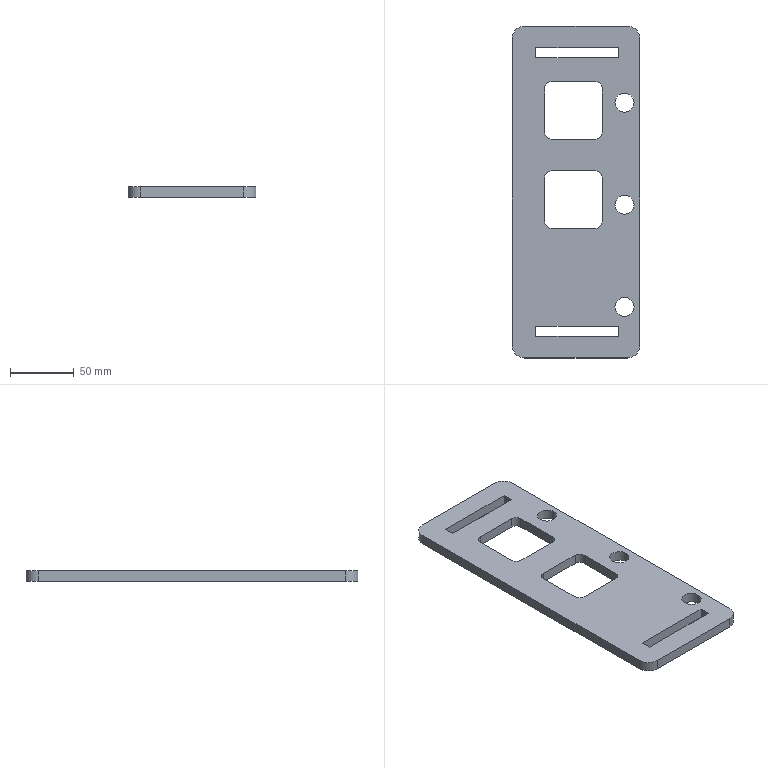Part | SolidWorks | features FlatPattern 1, SMBaseFlange 1, SheetMetal 1 | 1 solid | 40 faces | box 100 x 260 x 8 mm | volume 162695 mm3 | plane 22 | cylinder 18 | commonest cylinder face diameters 10 x8 15 x6 20 x4
STEP:
#1=CARTESIAN_POINT('',(-132.99,-115.,8.));
#2=VERTEX_POINT('',#1);
#3=CARTESIAN_POINT('',(-117.99,-115.,8.));
#4=VERTEX_POINT('',#3);
#5=CARTESIAN_POINT('',(-125.49,-115.,8.));
#6=DIRECTION('',(0.,0.,1.));
#7=DIRECTION('',(1.,0.,0.));
#8=AXIS2_PLACEMENT_3D('',#5,#6,#7);
#9=CIRCLE('',#8,7.5);
#10=EDGE_CURVE('',#2,#4,#9,.T.);
#11=ORIENTED_EDGE('',*,*,#10,.T.);
#12=CARTESIAN_POINT('',(-117.99,-115.,0.));
#13=VERTEX_POINT('',#12);
#14=CARTESIAN_POINT('',(-117.99,-115.,8.));
#15=DIRECTION('',(0.,0.,-1.));
#16=VECTOR('',#15,1000.);
#17=LINE('',#14,#16);
#18=EDGE_CURVE('',#4,#13,#17,.T.);
#19=ORIENTED_EDGE('',*,*,#18,.T.);
#20=CARTESIAN_POINT('',(-132.99,-115.,0.));
#21=VERTEX_POINT('',#20);
#22=CARTESIAN_POINT('',(-125.49,-115.,0.));
#23=DIRECTION('',(0.,0.,1.));
#24=DIRECTION('',(1.,0.,0.));
#25=AXIS2_PLACEMENT_3D('',#22,#23,#24);
#26=CIRCLE('',#25,7.5);
#27=EDGE_CURVE('',#21,#13,#26,.T.);
#28=ORIENTED_EDGE('',*,*,#27,.F.);
#29=CARTESIAN_POINT('',(-132.99,-115.,8.));
#30=DIRECTION('',(0.,0.,-1.));
#31=VECTOR('',#30,1000.);
#32=LINE('',#29,#31);
#33=EDGE_CURVE('',#2,#21,#32,.T.);
#34=ORIENTED_EDGE('',*,*,#33,.F.);
#35=EDGE_LOOP('',(#11,#19,#28,#34));
#36=FACE_OUTER_BOUND('',#35,.T.);
#37=CARTESIAN_POINT('',(-125.49,-115.,8.));
#38=DIRECTION('',(0.,0.,-1.));
#39=DIRECTION('',(-1.,0.,0.));
#40=AXIS2_PLACEMENT_3D('',#37,#38,#39);
#41=CYLINDRICAL_SURFACE('',#40,7.5);
#42=ADVANCED_FACE('',(#36),#41,.F.);
#43=CARTESIAN_POINT('',(-132.99,-195.,8.));
#44=VERTEX_POINT('',#43);
#45=CARTESIAN_POINT('',(-117.99,-195.,8.));
#46=VERTEX_POINT('',#45);
#47=CARTESIAN_POINT('',(-125.49,-195.,8.));
#48=DIRECTION('',(0.,0.,1.));
#49=DIRECTION('',(1.,0.,0.));
#50=AXIS2_PLACEMENT_3D('',#47,#48,#49);
#51=CIRCLE('',#50,7.5);
#52=EDGE_CURVE('',#44,#46,#51,.T.);
#53=ORIENTED_EDGE('',*,*,#52,.T.);
#54=CARTESIAN_POINT('',(-117.99,-195.,0.));
#55=VERTEX_POINT('',#54);
#56=CARTESIAN_POINT('',(-117.99,-195.,8.));
#57=DIRECTION('',(0.,0.,-1.));
#58=VECTOR('',#57,1000.);
#59=LINE('',#56,#58);
#60=EDGE_CURVE('',#46,#55,#59,.T.);
#61=ORIENTED_EDGE('',*,*,#60,.T.);
#62=CARTESIAN_POINT('',(-132.99,-195.,0.));
#63=VERTEX_POINT('',#62);
#64=CARTESIAN_POINT('',(-125.49,-195.,0.));
#65=DIRECTION('',(0.,0.,1.));
#66=DIRECTION('',(1.,0.,0.));
#67=AXIS2_PLACEMENT_3D('',#64,#65,#66);
#68=CIRCLE('',#67,7.5);
#69=EDGE_CURVE('',#63,#55,#68,.T.);
#70=ORIENTED_EDGE('',*,*,#69,.F.);
#71=CARTESIAN_POINT('',(-132.99,-195.,8.));
#72=DIRECTION('',(0.,0.,-1.));
#73=VECTOR('',#72,1000.);
#74=LINE('',#71,#73);
#75=EDGE_CURVE('',#44,#63,#74,.T.);
#76=ORIENTED_EDGE('',*,*,#75,.F.);
#77=EDGE_LOOP('',(#53,#61,#70,#76));
#78=FACE_OUTER_BOUND('',#77,.T.);
#79=CARTESIAN_POINT('',(-125.49,-195.,8.));
#80=DIRECTION('',(0.,0.,-1.));
#81=DIRECTION('',(-1.,0.,0.));
#82=AXIS2_PLACEMENT_3D('',#79,#80,#81);
#83=CYLINDRICAL_SURFACE('',#82,7.5);
#84=ADVANCED_FACE('',(#78),#83,.F.);
#85=CARTESIAN_POINT('',(-132.99,-275.,8.));
#86=VERTEX_POINT('',#85);
#87=CARTESIAN_POINT('',(-117.99,-275.,8.));
#88=VERTEX_POINT('',#87);
#89=CARTESIAN_POINT('',(-125.49,-275.,8.));
#90=DIRECTION('',(0.,0.,1.));
#91=DIRECTION('',(1.,0.,0.));
#92=AXIS2_PLACEMENT_3D('',#89,#90,#91);
#93=CIRCLE('',#92,7.5);
#94=EDGE_CURVE('',#86,#88,#93,.T.);
#95=ORIENTED_EDGE('',*,*,#94,.T.);
#96=CARTESIAN_POINT('',(-117.99,-275.,0.));
#97=VERTEX_POINT('',#96);
#98=CARTESIAN_POINT('',(-117.99,-275.,8.));
#99=DIRECTION('',(0.,0.,-1.));
#100=VECTOR('',#99,1000.);
#101=LINE('',#98,#100);
#102=EDGE_CURVE('',#88,#97,#101,.T.);
#103=ORIENTED_EDGE('',*,*,#102,.T.);
#104=CARTESIAN_POINT('',(-132.99,-275.,0.));
#105=VERTEX_POINT('',#104);
#106=CARTESIAN_POINT('',(-125.49,-275.,0.));
#107=DIRECTION('',(0.,0.,1.));
#108=DIRECTION('',(1.,0.,0.));
#109=AXIS2_PLACEMENT_3D('',#106,#107,#108);
#110=CIRCLE('',#109,7.5);
#111=EDGE_CURVE('',#105,#97,#110,.T.);
#112=ORIENTED_EDGE('',*,*,#111,.F.);
#113=CARTESIAN_POINT('',(-132.99,-275.,8.));
#114=DIRECTION('',(0.,0.,-1.));
#115=VECTOR('',#114,1000.);
#116=LINE('',#113,#115);
#117=EDGE_CURVE('',#86,#105,#116,.T.);
#118=ORIENTED_EDGE('',*,*,#117,.F.);
#119=EDGE_LOOP('',(#95,#103,#112,#118));
#120=FACE_OUTER_BOUND('',#119,.T.);
#121=CARTESIAN_POINT('',(-125.49,-275.,8.));
#122=DIRECTION('',(0.,0.,-1.));
#123=DIRECTION('',(-1.,0.,0.));
#124=AXIS2_PLACEMENT_3D('',#121,#122,#123);
#125=CYLINDRICAL_SURFACE('',#124,7.5);
#126=ADVANCED_FACE('',(#120),#125,.F.);
#127=ORIENTED_EDGE('',*,*,#52,.F.);
#128=CARTESIAN_POINT('',(-125.49,-195.,8.));
#129=DIRECTION('',(0.,0.,1.));
#130=DIRECTION('',(1.,0.,0.));
#131=AXIS2_PLACEMENT_3D('',#128,#129,#130);
#132=CIRCLE('',#131,7.5);
#133=EDGE_CURVE('',#46,#44,#132,.T.);
#134=ORIENTED_EDGE('',*,*,#133,.F.);
#135=EDGE_LOOP('',(#127,#134));
#136=FACE_BOUND('',#135,.T.);
#137=CARTESIAN_POINT('',(-213.472,-305.,8.));
#138=VERTEX_POINT('',#137);
#139=CARTESIAN_POINT('',(-203.472,-315.,8.));
#140=VERTEX_POINT('',#139);
#141=CARTESIAN_POINT('',(-203.472,-305.,8.));
#142=DIRECTION('',(0.,0.,1.));
#143=DIRECTION('',(1.,0.,0.));
#144=AXIS2_PLACEMENT_3D('',#141,#142,#143);
#145=CIRCLE('',#144,10.);
#146=EDGE_CURVE('',#138,#140,#145,.T.);
#147=ORIENTED_EDGE('',*,*,#146,.T.);
#148=CARTESIAN_POINT('',(-123.472,-315.,8.));
#149=VERTEX_POINT('',#148);
#150=CARTESIAN_POINT('',(-203.472,-315.,8.));
#151=DIRECTION('',(1.,0.,0.));
#152=VECTOR('',#151,1000.);
#153=LINE('',#150,#152);
#154=EDGE_CURVE('',#140,#149,#153,.T.);
#155=ORIENTED_EDGE('',*,*,#154,.T.);
#156=CARTESIAN_POINT('',(-113.472,-305.,8.));
#157=VERTEX_POINT('',#156);
#158=CARTESIAN_POINT('',(-123.472,-305.,8.));
#159=DIRECTION('',(0.,0.,1.));
#160=DIRECTION('',(1.,0.,0.));
#161=AXIS2_PLACEMENT_3D('',#158,#159,#160);
#162=CIRCLE('',#161,10.);
#163=EDGE_CURVE('',#149,#157,#162,.T.);
#164=ORIENTED_EDGE('',*,*,#163,.T.);
#165=CARTESIAN_POINT('',(-113.472,-65.,8.));
#166=VERTEX_POINT('',#165);
#167=CARTESIAN_POINT('',(-113.472,-65.,8.));
#168=DIRECTION('',(0.,1.,0.));
#169=VECTOR('',#168,1000.);
#170=LINE('',#167,#169);
#171=EDGE_CURVE('',#157,#166,#170,.T.);
#172=ORIENTED_EDGE('',*,*,#171,.T.);
#173=CARTESIAN_POINT('',(-123.472,-55.,8.));
#174=VERTEX_POINT('',#173);
#175=CARTESIAN_POINT('',(-123.472,-65.,8.));
#176=DIRECTION('',(0.,0.,1.));
#177=DIRECTION('',(-1.,0.,0.));
#178=AXIS2_PLACEMENT_3D('',#175,#176,#177);
#179=CIRCLE('',#178,10.);
#180=EDGE_CURVE('',#166,#174,#179,.T.);
#181=ORIENTED_EDGE('',*,*,#180,.T.);
#182=CARTESIAN_POINT('',(-203.472,-55.,8.));
#183=VERTEX_POINT('',#182);
#184=CARTESIAN_POINT('',(-203.472,-55.,8.));
#185=DIRECTION('',(-1.,0.,0.));
#186=VECTOR('',#185,1000.);
#187=LINE('',#184,#186);
#188=EDGE_CURVE('',#174,#183,#187,.T.);
#189=ORIENTED_EDGE('',*,*,#188,.T.);
#190=CARTESIAN_POINT('',(-213.472,-65.,8.));
#191=VERTEX_POINT('',#190);
#192=CARTESIAN_POINT('',(-203.472,-65.,8.));
#193=DIRECTION('',(0.,0.,1.));
#194=DIRECTION('',(1.,0.,0.));
#195=AXIS2_PLACEMENT_3D('',#192,#193,#194);
#196=CIRCLE('',#195,10.);
#197=EDGE_CURVE('',#183,#191,#196,.T.);
#198=ORIENTED_EDGE('',*,*,#197,.T.);
#199=CARTESIAN_POINT('',(-213.472,-65.,8.));
#200=DIRECTION('',(0.,-1.,0.));
#201=VECTOR('',#200,1000.);
#202=LINE('',#199,#201);
#203=EDGE_CURVE('',#191,#138,#202,.T.);
#204=ORIENTED_EDGE('',*,*,#203,.T.);
#205=EDGE_LOOP('',(#147,#155,#164,#172,#181,#189,#198,#204));
#206=FACE_OUTER_BOUND('',#205,.T.);
#207=ORIENTED_EDGE('',*,*,#94,.F.);
#208=CARTESIAN_POINT('',(-125.49,-275.,8.));
#209=DIRECTION('',(0.,0.,1.));
#210=DIRECTION('',(1.,0.,0.));
#211=AXIS2_PLACEMENT_3D('',#208,#209,#210);
#212=CIRCLE('',#211,7.5);
#213=EDGE_CURVE('',#88,#86,#212,.T.);
#214=ORIENTED_EDGE('',*,*,#213,.F.);
#215=EDGE_LOOP('',(#207,#214));
#216=FACE_BOUND('',#215,.T.);
#217=ORIENTED_EDGE('',*,*,#10,.F.);
#218=CARTESIAN_POINT('',(-125.49,-115.,8.));
#219=DIRECTION('',(0.,0.,1.));
#220=DIRECTION('',(1.,0.,0.));
#221=AXIS2_PLACEMENT_3D('',#218,#219,#220);
#222=CIRCLE('',#221,7.5);
#223=EDGE_CURVE('',#4,#2,#222,.T.);
#224=ORIENTED_EDGE('',*,*,#223,.F.);
#225=EDGE_LOOP('',(#217,#224));
#226=FACE_BOUND('',#225,.T.);
#227=CARTESIAN_POINT('',(-182.99,-143.5,8.));
#228=VERTEX_POINT('',#227);
#229=CARTESIAN_POINT('',(-147.99,-143.5,8.));
#230=VERTEX_POINT('',#229);
#231=CARTESIAN_POINT('',(-182.99,-143.5,8.));
#232=DIRECTION('',(1.,0.,0.));
#233=VECTOR('',#232,1000.);
#234=LINE('',#231,#233);
#235=EDGE_CURVE('',#228,#230,#234,.T.);
#236=ORIENTED_EDGE('',*,*,#235,.F.);
#237=CARTESIAN_POINT('',(-187.99,-138.5,8.));
#238=VERTEX_POINT('',#237);
#239=CARTESIAN_POINT('',(-182.99,-138.5,8.));
#240=DIRECTION('',(0.,0.,1.));
#241=DIRECTION('',(1.,0.,0.));
#242=AXIS2_PLACEMENT_3D('',#239,#240,#241);
#243=CIRCLE('',#242,5.);
#244=EDGE_CURVE('',#238,#228,#243,.T.);
#245=ORIENTED_EDGE('',*,*,#244,.F.);
#246=CARTESIAN_POINT('',(-187.99,-103.5,8.));
#247=VERTEX_POINT('',#246);
#248=CARTESIAN_POINT('',(-187.99,-103.5,8.));
#249=DIRECTION('',(0.,-1.,0.));
#250=VECTOR('',#249,1000.);
#251=LINE('',#248,#250);
#252=EDGE_CURVE('',#247,#238,#251,.T.);
#253=ORIENTED_EDGE('',*,*,#252,.F.);
#254=CARTESIAN_POINT('',(-182.99,-98.5,8.));
#255=VERTEX_POINT('',#254);
#256=CARTESIAN_POINT('',(-182.99,-103.5,8.));
#257=DIRECTION('',(0.,0.,1.));
#258=DIRECTION('',(1.,0.,0.));
#259=AXIS2_PLACEMENT_3D('',#256,#257,#258);
#260=CIRCLE('',#259,5.);
#261=EDGE_CURVE('',#255,#247,#260,.T.);
#262=ORIENTED_EDGE('',*,*,#261,.F.);
#263=CARTESIAN_POINT('',(-147.99,-98.5,8.));
#264=VERTEX_POINT('',#263);
#265=CARTESIAN_POINT('',(-182.99,-98.5,8.));
#266=DIRECTION('',(-1.,0.,0.));
#267=VECTOR('',#266,1000.);
#268=LINE('',#265,#267);
#269=EDGE_CURVE('',#264,#255,#268,.T.);
#270=ORIENTED_EDGE('',*,*,#269,.F.);
#271=CARTESIAN_POINT('',(-142.99,-103.5,8.));
#272=VERTEX_POINT('',#271);
#273=CARTESIAN_POINT('',(-147.99,-103.5,8.));
#274=DIRECTION('',(0.,0.,1.));
#275=DIRECTION('',(-1.,0.,0.));
#276=AXIS2_PLACEMENT_3D('',#273,#274,#275);
#277=CIRCLE('',#276,5.);
#278=EDGE_CURVE('',#272,#264,#277,.T.);
#279=ORIENTED_EDGE('',*,*,#278,.F.);
#280=CARTESIAN_POINT('',(-142.99,-138.5,8.));
#281=VERTEX_POINT('',#280);
#282=CARTESIAN_POINT('',(-142.99,-103.5,8.));
#283=DIRECTION('',(0.,1.,0.));
#284=VECTOR('',#283,1000.);
#285=LINE('',#282,#284);
#286=EDGE_CURVE('',#281,#272,#285,.T.);
#287=ORIENTED_EDGE('',*,*,#286,.F.);
#288=CARTESIAN_POINT('',(-147.99,-138.5,8.));
#289=DIRECTION('',(0.,0.,1.));
#290=DIRECTION('',(1.,0.,0.));
#291=AXIS2_PLACEMENT_3D('',#288,#289,#290);
#292=CIRCLE('',#291,5.);
#293=EDGE_CURVE('',#230,#281,#292,.T.);
#294=ORIENTED_EDGE('',*,*,#293,.F.);
#295=EDGE_LOOP('',(#236,#245,#253,#262,#270,#279,#287,#294));
#296=FACE_BOUND('',#295,.T.);
#297=CARTESIAN_POINT('',(-182.99,-213.5,8.));
#298=VERTEX_POINT('',#297);
#299=CARTESIAN_POINT('',(-147.99,-213.5,8.));
#300=VERTEX_POINT('',#299);
#301=CARTESIAN_POINT('',(-182.99,-213.5,8.));
#302=DIRECTION('',(1.,0.,0.));
#303=VECTOR('',#302,1000.);
#304=LINE('',#301,#303);
#305=EDGE_CURVE('',#298,#300,#304,.T.);
#306=ORIENTED_EDGE('',*,*,#305,.F.);
#307=CARTESIAN_POINT('',(-187.99,-208.5,8.));
#308=VERTEX_POINT('',#307);
#309=CARTESIAN_POINT('',(-182.99,-208.5,8.));
#310=DIRECTION('',(0.,0.,1.));
#311=DIRECTION('',(1.,0.,0.));
#312=AXIS2_PLACEMENT_3D('',#309,#310,#311);
#313=CIRCLE('',#312,5.);
#314=EDGE_CURVE('',#308,#298,#313,.T.);
#315=ORIENTED_EDGE('',*,*,#314,.F.);
#316=CARTESIAN_POINT('',(-187.99,-173.5,8.));
#317=VERTEX_POINT('',#316);
#318=CARTESIAN_POINT('',(-187.99,-173.5,8.));
#319=DIRECTION('',(0.,-1.,0.));
#320=VECTOR('',#319,1000.);
#321=LINE('',#318,#320);
#322=EDGE_CURVE('',#317,#308,#321,.T.);
#323=ORIENTED_EDGE('',*,*,#322,.F.);
#324=CARTESIAN_POINT('',(-182.99,-168.5,8.));
#325=VERTEX_POINT('',#324);
#326=CARTESIAN_POINT('',(-182.99,-173.5,8.));
#327=DIRECTION('',(0.,0.,1.));
#328=DIRECTION('',(1.,0.,0.));
#329=AXIS2_PLACEMENT_3D('',#326,#327,#328);
#330=CIRCLE('',#329,5.);
#331=EDGE_CURVE('',#325,#317,#330,.T.);
#332=ORIENTED_EDGE('',*,*,#331,.F.);
#333=CARTESIAN_POINT('',(-147.99,-168.5,8.));
#334=VERTEX_POINT('',#333);
#335=CARTESIAN_POINT('',(-182.99,-168.5,8.));
#336=DIRECTION('',(-1.,0.,0.));
#337=VECTOR('',#336,1000.);
#338=LINE('',#335,#337);
#339=EDGE_CURVE('',#334,#325,#338,.T.);
#340=ORIENTED_EDGE('',*,*,#339,.F.);
#341=CARTESIAN_POINT('',(-142.99,-173.5,8.));
#342=VERTEX_POINT('',#341);
#343=CARTESIAN_POINT('',(-147.99,-173.5,8.));
#344=DIRECTION('',(0.,0.,1.));
#345=DIRECTION('',(-1.,0.,0.));
#346=AXIS2_PLACEMENT_3D('',#343,#344,#345);
#347=CIRCLE('',#346,5.);
#348=EDGE_CURVE('',#342,#334,#347,.T.);
#349=ORIENTED_EDGE('',*,*,#348,.F.);
#350=CARTESIAN_POINT('',(-142.99,-208.5,8.));
#351=VERTEX_POINT('',#350);
#352=CARTESIAN_POINT('',(-142.99,-173.5,8.));
#353=DIRECTION('',(0.,1.,0.));
#354=VECTOR('',#353,1000.);
#355=LINE('',#352,#354);
#356=EDGE_CURVE('',#351,#342,#355,.T.);
#357=ORIENTED_EDGE('',*,*,#356,.F.);
#358=CARTESIAN_POINT('',(-147.99,-208.5,8.));
#359=DIRECTION('',(0.,0.,1.));
#360=DIRECTION('',(1.,0.,0.));
#361=AXIS2_PLACEMENT_3D('',#358,#359,#360);
#362=CIRCLE('',#361,5.);
#363=EDGE_CURVE('',#300,#351,#362,.T.);
#364=ORIENTED_EDGE('',*,*,#363,.F.);
#365=EDGE_LOOP('',(#306,#315,#323,#332,#340,#349,#357,#364));
#366=FACE_BOUND('',#365,.T.);
#367=CARTESIAN_POINT('',(-130.006,-290.,8.));
#368=VERTEX_POINT('',#367);
#369=CARTESIAN_POINT('',(-195.006,-290.,8.));
#370=VERTEX_POINT('',#369);
#371=CARTESIAN_POINT('',(-130.006,-290.,8.));
#372=DIRECTION('',(-1.,0.,0.));
#373=VECTOR('',#372,1000.);
#374=LINE('',#371,#373);
#375=EDGE_CURVE('',#368,#370,#374,.T.);
#376=ORIENTED_EDGE('',*,*,#375,.F.);
#377=CARTESIAN_POINT('',(-130.006,-298.,8.));
#378=VERTEX_POINT('',#377);
#379=CARTESIAN_POINT('',(-130.006,-298.,8.));
#380=DIRECTION('',(0.,1.,0.));
#381=VECTOR('',#380,1000.);
#382=LINE('',#379,#381);
#383=EDGE_CURVE('',#378,#368,#382,.T.);
#384=ORIENTED_EDGE('',*,*,#383,.F.);
#385=CARTESIAN_POINT('',(-195.006,-298.,8.));
#386=VERTEX_POINT('',#385);
#387=CARTESIAN_POINT('',(-130.006,-298.,8.));
#388=DIRECTION('',(1.,0.,0.));
#389=VECTOR('',#388,1000.);
#390=LINE('',#387,#389);
#391=EDGE_CURVE('',#386,#378,#390,.T.);
#392=ORIENTED_EDGE('',*,*,#391,.F.);
#393=CARTESIAN_POINT('',(-195.006,-298.,8.));
#394=DIRECTION('',(0.,-1.,0.));
#395=VECTOR('',#394,1000.);
#396=LINE('',#393,#395);
#397=EDGE_CURVE('',#370,#386,#396,.T.);
#398=ORIENTED_EDGE('',*,*,#397,.F.);
#399=EDGE_LOOP('',(#376,#384,#392,#398));
#400=FACE_BOUND('',#399,.T.);
#401=CARTESIAN_POINT('',(-130.006,-72.,8.));
#402=VERTEX_POINT('',#401);
#403=CARTESIAN_POINT('',(-195.006,-72.,8.));
#404=VERTEX_POINT('',#403);
#405=CARTESIAN_POINT('',(-130.006,-72.,8.));
#406=DIRECTION('',(-1.,0.,0.));
#407=VECTOR('',#406,1000.);
#408=LINE('',#405,#407);
#409=EDGE_CURVE('',#402,#404,#408,.T.);
#410=ORIENTED_EDGE('',*,*,#409,.F.);
#411=CARTESIAN_POINT('',(-130.006,-80.,8.));
#412=VERTEX_POINT('',#411);
#413=CARTESIAN_POINT('',(-130.006,-72.,8.));
#414=DIRECTION('',(0.,1.,0.));
#415=VECTOR('',#414,1000.);
#416=LINE('',#413,#415);
#417=EDGE_CURVE('',#412,#402,#416,.T.);
#418=ORIENTED_EDGE('',*,*,#417,.F.);
#419=CARTESIAN_POINT('',(-195.006,-80.,8.));
#420=VERTEX_POINT('',#419);
#421=CARTESIAN_POINT('',(-130.006,-80.,8.));
#422=DIRECTION('',(1.,0.,0.));
#423=VECTOR('',#422,1000.);
#424=LINE('',#421,#423);
#425=EDGE_CURVE('',#420,#412,#424,.T.);
#426=ORIENTED_EDGE('',*,*,#425,.F.);
#427=CARTESIAN_POINT('',(-195.006,-72.,8.));
#428=DIRECTION('',(0.,-1.,0.));
#429=VECTOR('',#428,1000.);
#430=LINE('',#427,#429);
#431=EDGE_CURVE('',#404,#420,#430,.T.);
#432=ORIENTED_EDGE('',*,*,#431,.F.);
#433=EDGE_LOOP('',(#410,#418,#426,#432));
#434=FACE_BOUND('',#433,.T.);
#435=CARTESIAN_POINT('',(-203.472,-305.,8.));
#436=DIRECTION('',(0.,0.,1.));
#437=DIRECTION('',(1.,0.,0.));
#438=AXIS2_PLACEMENT_3D('',#435,#436,#437);
#439=PLANE('',#438);
#440=ADVANCED_FACE('',(#136,#206,#216,#226,#296,#366,#400,#434),#439,.T.);
#441=CARTESIAN_POINT('',(-130.006,-298.,0.));
#442=VERTEX_POINT('',#441);
#443=CARTESIAN_POINT('',(-130.006,-290.,0.));
#444=VERTEX_POINT('',#443);
#445=CARTESIAN_POINT('',(-130.006,-298.,0.));
#446=DIRECTION('',(0.,1.,0.));
#447=VECTOR('',#446,1000.);
#448=LINE('',#445,#447);
#449=EDGE_CURVE('',#442,#444,#448,.T.);
#450=ORIENTED_EDGE('',*,*,#449,.T.);
#451=CARTESIAN_POINT('',(-195.006,-290.,0.));
#452=VERTEX_POINT('',#451);
#453=CARTESIAN_POINT('',(-130.006,-290.,0.));
#454=DIRECTION('',(-1.,0.,0.));
#455=VECTOR('',#454,1000.);
#456=LINE('',#453,#455);
#457=EDGE_CURVE('',#444,#452,#456,.T.);
#458=ORIENTED_EDGE('',*,*,#457,.T.);
#459=CARTESIAN_POINT('',(-195.006,-298.,0.));
#460=VERTEX_POINT('',#459);
#461=CARTESIAN_POINT('',(-195.006,-298.,0.));
#462=DIRECTION('',(0.,-1.,0.));
#463=VECTOR('',#462,1000.);
#464=LINE('',#461,#463);
#465=EDGE_CURVE('',#452,#460,#464,.T.);
#466=ORIENTED_EDGE('',*,*,#465,.T.);
#467=CARTESIAN_POINT('',(-130.006,-298.,0.));
#468=DIRECTION('',(1.,0.,0.));
#469=VECTOR('',#468,1000.);
#470=LINE('',#467,#469);
#471=EDGE_CURVE('',#460,#442,#470,.T.);
#472=ORIENTED_EDGE('',*,*,#471,.T.);
#473=EDGE_LOOP('',(#450,#458,#466,#472));
#474=FACE_BOUND('',#473,.T.);
#475=CARTESIAN_POINT('',(-187.99,-138.5,0.));
#476=VERTEX_POINT('',#475);
#477=CARTESIAN_POINT('',(-182.99,-143.5,0.));
#478=VERTEX_POINT('',#477);
#479=CARTESIAN_POINT('',(-182.99,-138.5,0.));
#480=DIRECTION('',(0.,0.,1.));
#481=DIRECTION('',(1.,0.,0.));
#482=AXIS2_PLACEMENT_3D('',#479,#480,#481);
#483=CIRCLE('',#482,5.);
#484=EDGE_CURVE('',#476,#478,#483,.T.);
#485=ORIENTED_EDGE('',*,*,#484,.T.);
#486=CARTESIAN_POINT('',(-147.99,-143.5,0.));
#487=VERTEX_POINT('',#486);
#488=CARTESIAN_POINT('',(-182.99,-143.5,0.));
#489=DIRECTION('',(1.,0.,0.));
#490=VECTOR('',#489,1000.);
#491=LINE('',#488,#490);
#492=EDGE_CURVE('',#478,#487,#491,.T.);
#493=ORIENTED_EDGE('',*,*,#492,.T.);
#494=CARTESIAN_POINT('',(-142.99,-138.5,0.));
#495=VERTEX_POINT('',#494);
#496=CARTESIAN_POINT('',(-147.99,-138.5,0.));
#497=DIRECTION('',(0.,0.,1.));
#498=DIRECTION('',(1.,0.,0.));
#499=AXIS2_PLACEMENT_3D('',#496,#497,#498);
#500=CIRCLE('',#499,5.);
#501=EDGE_CURVE('',#487,#495,#500,.T.);
#502=ORIENTED_EDGE('',*,*,#501,.T.);
#503=CARTESIAN_POINT('',(-142.99,-103.5,0.));
#504=VERTEX_POINT('',#503);
#505=CARTESIAN_POINT('',(-142.99,-103.5,0.));
#506=DIRECTION('',(0.,1.,0.));
#507=VECTOR('',#506,1000.);
#508=LINE('',#505,#507);
#509=EDGE_CURVE('',#495,#504,#508,.T.);
#510=ORIENTED_EDGE('',*,*,#509,.T.);
#511=CARTESIAN_POINT('',(-147.99,-98.5,0.));
#512=VERTEX_POINT('',#511);
#513=CARTESIAN_POINT('',(-147.99,-103.5,0.));
#514=DIRECTION('',(0.,0.,1.));
#515=DIRECTION('',(-1.,0.,0.));
#516=AXIS2_PLACEMENT_3D('',#513,#514,#515);
#517=CIRCLE('',#516,5.);
#518=EDGE_CURVE('',#504,#512,#517,.T.);
#519=ORIENTED_EDGE('',*,*,#518,.T.);
#520=CARTESIAN_POINT('',(-182.99,-98.5,0.));
#521=VERTEX_POINT('',#520);
#522=CARTESIAN_POINT('',(-182.99,-98.5,0.));
#523=DIRECTION('',(-1.,0.,0.));
#524=VECTOR('',#523,1000.);
#525=LINE('',#522,#524);
#526=EDGE_CURVE('',#512,#521,#525,.T.);
#527=ORIENTED_EDGE('',*,*,#526,.T.);
#528=CARTESIAN_POINT('',(-187.99,-103.5,0.));
#529=VERTEX_POINT('',#528);
#530=CARTESIAN_POINT('',(-182.99,-103.5,0.));
#531=DIRECTION('',(0.,0.,1.));
#532=DIRECTION('',(1.,0.,0.));
#533=AXIS2_PLACEMENT_3D('',#530,#531,#532);
#534=CIRCLE('',#533,5.);
#535=EDGE_CURVE('',#521,#529,#534,.T.);
#536=ORIENTED_EDGE('',*,*,#535,.T.);
#537=CARTESIAN_POINT('',(-187.99,-103.5,0.));
#538=DIRECTION('',(0.,-1.,0.));
#539=VECTOR('',#538,1000.);
#540=LINE('',#537,#539);
#541=EDGE_CURVE('',#529,#476,#540,.T.);
#542=ORIENTED_EDGE('',*,*,#541,.T.);
#543=EDGE_LOOP('',(#485,#493,#502,#510,#519,#527,#536,#542));
#544=FACE_BOUND('',#543,.T.);
#545=CARTESIAN_POINT('',(-213.472,-305.,0.));
#546=VERTEX_POINT('',#545);
#547=CARTESIAN_POINT('',(-203.472,-315.,0.));
#548=VERTEX_POINT('',#547);
#549=CARTESIAN_POINT('',(-203.472,-305.,0.));
#550=DIRECTION('',(0.,0.,1.));
#551=DIRECTION('',(1.,0.,0.));
#552=AXIS2_PLACEMENT_3D('',#549,#550,#551);
#553=CIRCLE('',#552,10.);
#554=EDGE_CURVE('',#546,#548,#553,.T.);
#555=ORIENTED_EDGE('',*,*,#554,.F.);
#556=CARTESIAN_POINT('',(-213.472,-65.,0.));
#557=VERTEX_POINT('',#556);
#558=CARTESIAN_POINT('',(-213.472,-65.,0.));
#559=DIRECTION('',(0.,-1.,0.));
#560=VECTOR('',#559,1000.);
#561=LINE('',#558,#560);
#562=EDGE_CURVE('',#557,#546,#561,.T.);
#563=ORIENTED_EDGE('',*,*,#562,.F.);
#564=CARTESIAN_POINT('',(-203.472,-55.,0.));
#565=VERTEX_POINT('',#564);
#566=CARTESIAN_POINT('',(-203.472,-65.,0.));
#567=DIRECTION('',(0.,0.,1.));
#568=DIRECTION('',(1.,0.,0.));
#569=AXIS2_PLACEMENT_3D('',#566,#567,#568);
#570=CIRCLE('',#569,10.);
#571=EDGE_CURVE('',#565,#557,#570,.T.);
#572=ORIENTED_EDGE('',*,*,#571,.F.);
#573=CARTESIAN_POINT('',(-123.472,-55.,0.));
#574=VERTEX_POINT('',#573);
#575=CARTESIAN_POINT('',(-203.472,-55.,0.));
#576=DIRECTION('',(-1.,0.,0.));
#577=VECTOR('',#576,1000.);
#578=LINE('',#575,#577);
#579=EDGE_CURVE('',#574,#565,#578,.T.);
#580=ORIENTED_EDGE('',*,*,#579,.F.);
#581=CARTESIAN_POINT('',(-113.472,-65.,0.));
#582=VERTEX_POINT('',#581);
#583=CARTESIAN_POINT('',(-123.472,-65.,0.));
#584=DIRECTION('',(0.,0.,1.));
#585=DIRECTION('',(-1.,0.,0.));
#586=AXIS2_PLACEMENT_3D('',#583,#584,#585);
#587=CIRCLE('',#586,10.);
#588=EDGE_CURVE('',#582,#574,#587,.T.);
#589=ORIENTED_EDGE('',*,*,#588,.F.);
#590=CARTESIAN_POINT('',(-113.472,-305.,0.));
#591=VERTEX_POINT('',#590);
#592=CARTESIAN_POINT('',(-113.472,-65.,0.));
#593=DIRECTION('',(0.,1.,0.));
#594=VECTOR('',#593,1000.);
#595=LINE('',#592,#594);
#596=EDGE_CURVE('',#591,#582,#595,.T.);
#597=ORIENTED_EDGE('',*,*,#596,.F.);
#598=CARTESIAN_POINT('',(-123.472,-315.,0.));
#599=VERTEX_POINT('',#598);
#600=CARTESIAN_POINT('',(-123.472,-305.,0.));
#601=DIRECTION('',(0.,0.,1.));
#602=DIRECTION('',(1.,0.,0.));
#603=AXIS2_PLACEMENT_3D('',#600,#601,#602);
#604=CIRCLE('',#603,10.);
#605=EDGE_CURVE('',#599,#591,#604,.T.);
#606=ORIENTED_EDGE('',*,*,#605,.F.);
#607=CARTESIAN_POINT('',(-203.472,-315.,0.));
#608=DIRECTION('',(1.,0.,0.));
#609=VECTOR('',#608,1000.);
#610=LINE('',#607,#609);
#611=EDGE_CURVE('',#548,#599,#610,.T.);
#612=ORIENTED_EDGE('',*,*,#611,.F.);
#613=EDGE_LOOP('',(#555,#563,#572,#580,#589,#597,#606,#612));
#614=FACE_OUTER_BOUND('',#613,.T.);
#615=ORIENTED_EDGE('',*,*,#111,.T.);
#616=CARTESIAN_POINT('',(-125.49,-275.,0.));
#617=DIRECTION('',(0.,0.,1.));
#618=DIRECTION('',(1.,0.,0.));
#619=AXIS2_PLACEMENT_3D('',#616,#617,#618);
#620=CIRCLE('',#619,7.5);
#621=EDGE_CURVE('',#97,#105,#620,.T.);
#622=ORIENTED_EDGE('',*,*,#621,.T.);
#623=EDGE_LOOP('',(#615,#622));
#624=FACE_BOUND('',#623,.T.);
#625=ORIENTED_EDGE('',*,*,#69,.T.);
#626=CARTESIAN_POINT('',(-125.49,-195.,0.));
#627=DIRECTION('',(0.,0.,1.));
#628=DIRECTION('',(1.,0.,0.));
#629=AXIS2_PLACEMENT_3D('',#626,#627,#628);
#630=CIRCLE('',#629,7.5);
#631=EDGE_CURVE('',#55,#63,#630,.T.);
#632=ORIENTED_EDGE('',*,*,#631,.T.);
#633=EDGE_LOOP('',(#625,#632));
#634=FACE_BOUND('',#633,.T.);
#635=ORIENTED_EDGE('',*,*,#27,.T.);
#636=CARTESIAN_POINT('',(-125.49,-115.,0.));
#637=DIRECTION('',(0.,0.,1.));
#638=DIRECTION('',(1.,0.,0.));
#639=AXIS2_PLACEMENT_3D('',#636,#637,#638);
#640=CIRCLE('',#639,7.5);
#641=EDGE_CURVE('',#13,#21,#640,.T.);
#642=ORIENTED_EDGE('',*,*,#641,.T.);
#643=EDGE_LOOP('',(#635,#642));
#644=FACE_BOUND('',#643,.T.);
#645=CARTESIAN_POINT('',(-187.99,-208.5,0.));
#646=VERTEX_POINT('',#645);
#647=CARTESIAN_POINT('',(-182.99,-213.5,0.));
#648=VERTEX_POINT('',#647);
#649=CARTESIAN_POINT('',(-182.99,-208.5,0.));
#650=DIRECTION('',(0.,0.,1.));
#651=DIRECTION('',(1.,0.,0.));
#652=AXIS2_PLACEMENT_3D('',#649,#650,#651);
#653=CIRCLE('',#652,5.);
#654=EDGE_CURVE('',#646,#648,#653,.T.);
#655=ORIENTED_EDGE('',*,*,#654,.T.);
#656=CARTESIAN_POINT('',(-147.99,-213.5,0.));
#657=VERTEX_POINT('',#656);
#658=CARTESIAN_POINT('',(-182.99,-213.5,0.));
#659=DIRECTION('',(1.,0.,0.));
#660=VECTOR('',#659,1000.);
#661=LINE('',#658,#660);
#662=EDGE_CURVE('',#648,#657,#661,.T.);
#663=ORIENTED_EDGE('',*,*,#662,.T.);
#664=CARTESIAN_POINT('',(-142.99,-208.5,0.));
#665=VERTEX_POINT('',#664);
#666=CARTESIAN_POINT('',(-147.99,-208.5,0.));
#667=DIRECTION('',(0.,0.,1.));
#668=DIRECTION('',(1.,0.,0.));
#669=AXIS2_PLACEMENT_3D('',#666,#667,#668);
#670=CIRCLE('',#669,5.);
#671=EDGE_CURVE('',#657,#665,#670,.T.);
#672=ORIENTED_EDGE('',*,*,#671,.T.);
#673=CARTESIAN_POINT('',(-142.99,-173.5,0.));
#674=VERTEX_POINT('',#673);
#675=CARTESIAN_POINT('',(-142.99,-173.5,0.));
#676=DIRECTION('',(0.,1.,0.));
#677=VECTOR('',#676,1000.);
#678=LINE('',#675,#677);
#679=EDGE_CURVE('',#665,#674,#678,.T.);
#680=ORIENTED_EDGE('',*,*,#679,.T.);
#681=CARTESIAN_POINT('',(-147.99,-168.5,0.));
#682=VERTEX_POINT('',#681);
#683=CARTESIAN_POINT('',(-147.99,-173.5,0.));
#684=DIRECTION('',(0.,0.,1.));
#685=DIRECTION('',(-1.,0.,0.));
#686=AXIS2_PLACEMENT_3D('',#683,#684,#685);
#687=CIRCLE('',#686,5.);
#688=EDGE_CURVE('',#674,#682,#687,.T.);
#689=ORIENTED_EDGE('',*,*,#688,.T.);
#690=CARTESIAN_POINT('',(-182.99,-168.5,0.));
#691=VERTEX_POINT('',#690);
#692=CARTESIAN_POINT('',(-182.99,-168.5,0.));
#693=DIRECTION('',(-1.,0.,0.));
#694=VECTOR('',#693,1000.);
#695=LINE('',#692,#694);
#696=EDGE_CURVE('',#682,#691,#695,.T.);
#697=ORIENTED_EDGE('',*,*,#696,.T.);
#698=CARTESIAN_POINT('',(-187.99,-173.5,0.));
#699=VERTEX_POINT('',#698);
#700=CARTESIAN_POINT('',(-182.99,-173.5,0.));
#701=DIRECTION('',(0.,0.,1.));
#702=DIRECTION('',(1.,0.,0.));
#703=AXIS2_PLACEMENT_3D('',#700,#701,#702);
#704=CIRCLE('',#703,5.);
#705=EDGE_CURVE('',#691,#699,#704,.T.);
#706=ORIENTED_EDGE('',*,*,#705,.T.);
#707=CARTESIAN_POINT('',(-187.99,-173.5,0.));
#708=DIRECTION('',(0.,-1.,0.));
#709=VECTOR('',#708,1000.);
#710=LINE('',#707,#709);
#711=EDGE_CURVE('',#699,#646,#710,.T.);
#712=ORIENTED_EDGE('',*,*,#711,.T.);
#713=EDGE_LOOP('',(#655,#663,#672,#680,#689,#697,#706,#712));
#714=FACE_BOUND('',#713,.T.);
#715=CARTESIAN_POINT('',(-130.006,-80.,0.));
#716=VERTEX_POINT('',#715);
#717=CARTESIAN_POINT('',(-130.006,-72.,0.));
#718=VERTEX_POINT('',#717);
#719=CARTESIAN_POINT('',(-130.006,-72.,0.));
#720=DIRECTION('',(0.,1.,0.));
#721=VECTOR('',#720,1000.);
#722=LINE('',#719,#721);
#723=EDGE_CURVE('',#716,#718,#722,.T.);
#724=ORIENTED_EDGE('',*,*,#723,.T.);
#725=CARTESIAN_POINT('',(-195.006,-72.,0.));
#726=VERTEX_POINT('',#725);
#727=CARTESIAN_POINT('',(-130.006,-72.,0.));
#728=DIRECTION('',(-1.,0.,0.));
#729=VECTOR('',#728,1000.);
#730=LINE('',#727,#729);
#731=EDGE_CURVE('',#718,#726,#730,.T.);
#732=ORIENTED_EDGE('',*,*,#731,.T.);
#733=CARTESIAN_POINT('',(-195.006,-80.,0.));
#734=VERTEX_POINT('',#733);
#735=CARTESIAN_POINT('',(-195.006,-72.,0.));
#736=DIRECTION('',(0.,-1.,0.));
#737=VECTOR('',#736,1000.);
#738=LINE('',#735,#737);
#739=EDGE_CURVE('',#726,#734,#738,.T.);
#740=ORIENTED_EDGE('',*,*,#739,.T.);
#741=CARTESIAN_POINT('',(-130.006,-80.,0.));
#742=DIRECTION('',(1.,0.,0.));
#743=VECTOR('',#742,1000.);
#744=LINE('',#741,#743);
#745=EDGE_CURVE('',#734,#716,#744,.T.);
#746=ORIENTED_EDGE('',*,*,#745,.T.);
#747=EDGE_LOOP('',(#724,#732,#740,#746));
#748=FACE_BOUND('',#747,.T.);
#749=CARTESIAN_POINT('',(-203.472,-305.,0.));
#750=DIRECTION('',(0.,0.,1.));
#751=DIRECTION('',(1.,0.,0.));
#752=AXIS2_PLACEMENT_3D('',#749,#750,#751);
#753=PLANE('',#752);
#754=ADVANCED_FACE('',(#474,#544,#614,#624,#634,#644,#714,#748),#753,.F.);
#755=ORIENTED_EDGE('',*,*,#554,.T.);
#756=CARTESIAN_POINT('',(-203.472,-315.,8.));
#757=DIRECTION('',(0.,0.,-1.));
#758=VECTOR('',#757,1000.);
#759=LINE('',#756,#758);
#760=EDGE_CURVE('',#140,#548,#759,.T.);
#761=ORIENTED_EDGE('',*,*,#760,.F.);
#762=ORIENTED_EDGE('',*,*,#146,.F.);
#763=CARTESIAN_POINT('',(-213.472,-305.,8.));
#764=DIRECTION('',(0.,0.,-1.));
#765=VECTOR('',#764,1000.);
#766=LINE('',#763,#765);
#767=EDGE_CURVE('',#138,#546,#766,.T.);
#768=ORIENTED_EDGE('',*,*,#767,.T.);
#769=EDGE_LOOP('',(#755,#761,#762,#768));
#770=FACE_OUTER_BOUND('',#769,.T.);
#771=CARTESIAN_POINT('',(-203.472,-305.,8.));
#772=DIRECTION('',(0.,0.,-1.));
#773=DIRECTION('',(-1.,0.,0.));
#774=AXIS2_PLACEMENT_3D('',#771,#772,#773);
#775=CYLINDRICAL_SURFACE('',#774,10.);
#776=ADVANCED_FACE('',(#770),#775,.T.);
#777=ORIENTED_EDGE('',*,*,#611,.T.);
#778=CARTESIAN_POINT('',(-123.472,-315.,8.));
#779=DIRECTION('',(0.,0.,-1.));
#780=VECTOR('',#779,1000.);
#781=LINE('',#778,#780);
#782=EDGE_CURVE('',#149,#599,#781,.T.);
#783=ORIENTED_EDGE('',*,*,#782,.F.);
#784=ORIENTED_EDGE('',*,*,#154,.F.);
#785=ORIENTED_EDGE('',*,*,#760,.T.);
#786=EDGE_LOOP('',(#777,#783,#784,#785));
#787=FACE_OUTER_BOUND('',#786,.T.);
#788=CARTESIAN_POINT('',(-203.472,-315.,8.));
#789=DIRECTION('',(0.,1.,0.));
#790=DIRECTION('',(0.,0.,1.));
#791=AXIS2_PLACEMENT_3D('',#788,#789,#790);
#792=PLANE('',#791);
#793=ADVANCED_FACE('',(#787),#792,.F.);
#794=ORIENTED_EDGE('',*,*,#605,.T.);
#795=CARTESIAN_POINT('',(-113.472,-305.,8.));
#796=DIRECTION('',(0.,0.,-1.));
#797=VECTOR('',#796,1000.);
#798=LINE('',#795,#797);
#799=EDGE_CURVE('',#157,#591,#798,.T.);
#800=ORIENTED_EDGE('',*,*,#799,.F.);
#801=ORIENTED_EDGE('',*,*,#163,.F.);
#802=ORIENTED_EDGE('',*,*,#782,.T.);
#803=EDGE_LOOP('',(#794,#800,#801,#802));
#804=FACE_OUTER_BOUND('',#803,.T.);
#805=CARTESIAN_POINT('',(-123.472,-305.,8.));
#806=DIRECTION('',(0.,0.,-1.));
#807=DIRECTION('',(-1.,0.,0.));
#808=AXIS2_PLACEMENT_3D('',#805,#806,#807);
#809=CYLINDRICAL_SURFACE('',#808,10.);
#810=ADVANCED_FACE('',(#804),#809,.T.);
#811=ORIENTED_EDGE('',*,*,#596,.T.);
#812=CARTESIAN_POINT('',(-113.472,-65.,8.));
#813=DIRECTION('',(0.,0.,-1.));
#814=VECTOR('',#813,1000.);
#815=LINE('',#812,#814);
#816=EDGE_CURVE('',#166,#582,#815,.T.);
#817=ORIENTED_EDGE('',*,*,#816,.F.);
#818=ORIENTED_EDGE('',*,*,#171,.F.);
#819=ORIENTED_EDGE('',*,*,#799,.T.);
#820=EDGE_LOOP('',(#811,#817,#818,#819));
#821=FACE_OUTER_BOUND('',#820,.T.);
#822=CARTESIAN_POINT('',(-113.472,-65.,8.));
#823=DIRECTION('',(-1.,0.,0.));
#824=DIRECTION('',(0.,-1.,0.));
#825=AXIS2_PLACEMENT_3D('',#822,#823,#824);
#826=PLANE('',#825);
#827=ADVANCED_FACE('',(#821),#826,.F.);
#828=ORIENTED_EDGE('',*,*,#588,.T.);
#829=CARTESIAN_POINT('',(-123.472,-55.,8.));
#830=DIRECTION('',(0.,0.,-1.));
#831=VECTOR('',#830,1000.);
#832=LINE('',#829,#831);
#833=EDGE_CURVE('',#174,#574,#832,.T.);
#834=ORIENTED_EDGE('',*,*,#833,.F.);
#835=ORIENTED_EDGE('',*,*,#180,.F.);
#836=ORIENTED_EDGE('',*,*,#816,.T.);
#837=EDGE_LOOP('',(#828,#834,#835,#836));
#838=FACE_OUTER_BOUND('',#837,.T.);
#839=CARTESIAN_POINT('',(-123.472,-65.,8.));
#840=DIRECTION('',(0.,0.,-1.));
#841=DIRECTION('',(-1.,0.,0.));
#842=AXIS2_PLACEMENT_3D('',#839,#840,#841);
#843=CYLINDRICAL_SURFACE('',#842,10.);
#844=ADVANCED_FACE('',(#838),#843,.T.);
#845=ORIENTED_EDGE('',*,*,#579,.T.);
#846=CARTESIAN_POINT('',(-203.472,-55.,8.));
#847=DIRECTION('',(0.,0.,-1.));
#848=VECTOR('',#847,1000.);
#849=LINE('',#846,#848);
#850=EDGE_CURVE('',#183,#565,#849,.T.);
#851=ORIENTED_EDGE('',*,*,#850,.F.);
#852=ORIENTED_EDGE('',*,*,#188,.F.);
#853=ORIENTED_EDGE('',*,*,#833,.T.);
#854=EDGE_LOOP('',(#845,#851,#852,#853));
#855=FACE_OUTER_BOUND('',#854,.T.);
#856=CARTESIAN_POINT('',(-203.472,-55.,8.));
#857=DIRECTION('',(0.,-1.,0.));
#858=DIRECTION('',(1.,0.,0.));
#859=AXIS2_PLACEMENT_3D('',#856,#857,#858);
#860=PLANE('',#859);
#861=ADVANCED_FACE('',(#855),#860,.F.);
#862=ORIENTED_EDGE('',*,*,#571,.T.);
#863=CARTESIAN_POINT('',(-213.472,-65.,8.));
#864=DIRECTION('',(0.,0.,-1.));
#865=VECTOR('',#864,1000.);
#866=LINE('',#863,#865);
#867=EDGE_CURVE('',#191,#557,#866,.T.);
#868=ORIENTED_EDGE('',*,*,#867,.F.);
#869=ORIENTED_EDGE('',*,*,#197,.F.);
#870=ORIENTED_EDGE('',*,*,#850,.T.);
#871=EDGE_LOOP('',(#862,#868,#869,#870));
#872=FACE_OUTER_BOUND('',#871,.T.);
#873=CARTESIAN_POINT('',(-203.472,-65.,8.));
#874=DIRECTION('',(0.,0.,-1.));
#875=DIRECTION('',(-1.,0.,0.));
#876=AXIS2_PLACEMENT_3D('',#873,#874,#875);
#877=CYLINDRICAL_SURFACE('',#876,10.);
#878=ADVANCED_FACE('',(#872),#877,.T.);
#879=ORIENTED_EDGE('',*,*,#562,.T.);
#880=ORIENTED_EDGE('',*,*,#767,.F.);
#881=ORIENTED_EDGE('',*,*,#203,.F.);
#882=ORIENTED_EDGE('',*,*,#867,.T.);
#883=EDGE_LOOP('',(#879,#880,#881,#882));
#884=FACE_OUTER_BOUND('',#883,.T.);
#885=CARTESIAN_POINT('',(-213.472,-65.,8.));
#886=DIRECTION('',(1.,0.,0.));
#887=DIRECTION('',(0.,1.,0.));
#888=AXIS2_PLACEMENT_3D('',#885,#886,#887);
#889=PLANE('',#888);
#890=ADVANCED_FACE('',(#884),#889,.F.);
#891=ORIENTED_EDGE('',*,*,#102,.F.);
#892=ORIENTED_EDGE('',*,*,#213,.T.);
#893=ORIENTED_EDGE('',*,*,#117,.T.);
#894=ORIENTED_EDGE('',*,*,#621,.F.);
#895=EDGE_LOOP('',(#891,#892,#893,#894));
#896=FACE_OUTER_BOUND('',#895,.T.);
#897=CARTESIAN_POINT('',(-125.49,-275.,8.));
#898=DIRECTION('',(0.,0.,-1.));
#899=DIRECTION('',(-1.,0.,0.));
#900=AXIS2_PLACEMENT_3D('',#897,#898,#899);
#901=CYLINDRICAL_SURFACE('',#900,7.5);
#902=ADVANCED_FACE('',(#896),#901,.F.);
#903=ORIENTED_EDGE('',*,*,#60,.F.);
#904=ORIENTED_EDGE('',*,*,#133,.T.);
#905=ORIENTED_EDGE('',*,*,#75,.T.);
#906=ORIENTED_EDGE('',*,*,#631,.F.);
#907=EDGE_LOOP('',(#903,#904,#905,#906));
#908=FACE_OUTER_BOUND('',#907,.T.);
#909=CARTESIAN_POINT('',(-125.49,-195.,8.));
#910=DIRECTION('',(0.,0.,-1.));
#911=DIRECTION('',(-1.,0.,0.));
#912=AXIS2_PLACEMENT_3D('',#909,#910,#911);
#913=CYLINDRICAL_SURFACE('',#912,7.5);
#914=ADVANCED_FACE('',(#908),#913,.F.);
#915=ORIENTED_EDGE('',*,*,#18,.F.);
#916=ORIENTED_EDGE('',*,*,#223,.T.);
#917=ORIENTED_EDGE('',*,*,#33,.T.);
#918=ORIENTED_EDGE('',*,*,#641,.F.);
#919=EDGE_LOOP('',(#915,#916,#917,#918));
#920=FACE_OUTER_BOUND('',#919,.T.);
#921=CARTESIAN_POINT('',(-125.49,-115.,8.));
#922=DIRECTION('',(0.,0.,-1.));
#923=DIRECTION('',(-1.,0.,0.));
#924=AXIS2_PLACEMENT_3D('',#921,#922,#923);
#925=CYLINDRICAL_SURFACE('',#924,7.5);
#926=ADVANCED_FACE('',(#920),#925,.F.);
#927=ORIENTED_EDGE('',*,*,#484,.F.);
#928=CARTESIAN_POINT('',(-187.99,-138.5,8.));
#929=DIRECTION('',(0.,0.,-1.));
#930=VECTOR('',#929,1000.);
#931=LINE('',#928,#930);
#932=EDGE_CURVE('',#238,#476,#931,.T.);
#933=ORIENTED_EDGE('',*,*,#932,.F.);
#934=ORIENTED_EDGE('',*,*,#244,.T.);
#935=CARTESIAN_POINT('',(-182.99,-143.5,8.));
#936=DIRECTION('',(0.,0.,-1.));
#937=VECTOR('',#936,1000.);
#938=LINE('',#935,#937);
#939=EDGE_CURVE('',#228,#478,#938,.T.);
#940=ORIENTED_EDGE('',*,*,#939,.T.);
#941=EDGE_LOOP('',(#927,#933,#934,#940));
#942=FACE_OUTER_BOUND('',#941,.T.);
#943=CARTESIAN_POINT('',(-182.99,-138.5,8.));
#944=DIRECTION('',(0.,0.,-1.));
#945=DIRECTION('',(-1.,0.,0.));
#946=AXIS2_PLACEMENT_3D('',#943,#944,#945);
#947=CYLINDRICAL_SURFACE('',#946,5.);
#948=ADVANCED_FACE('',(#942),#947,.F.);
#949=ORIENTED_EDGE('',*,*,#492,.F.);
#950=ORIENTED_EDGE('',*,*,#939,.F.);
#951=ORIENTED_EDGE('',*,*,#235,.T.);
#952=CARTESIAN_POINT('',(-147.99,-143.5,8.));
#953=DIRECTION('',(0.,0.,-1.));
#954=VECTOR('',#953,1000.);
#955=LINE('',#952,#954);
#956=EDGE_CURVE('',#230,#487,#955,.T.);
#957=ORIENTED_EDGE('',*,*,#956,.T.);
#958=EDGE_LOOP('',(#949,#950,#951,#957));
#959=FACE_OUTER_BOUND('',#958,.T.);
#960=CARTESIAN_POINT('',(-182.99,-143.5,8.));
#961=DIRECTION('',(0.,1.,0.));
#962=DIRECTION('',(0.,0.,1.));
#963=AXIS2_PLACEMENT_3D('',#960,#961,#962);
#964=PLANE('',#963);
#965=ADVANCED_FACE('',(#959),#964,.T.);
#966=ORIENTED_EDGE('',*,*,#501,.F.);
#967=ORIENTED_EDGE('',*,*,#956,.F.);
#968=ORIENTED_EDGE('',*,*,#293,.T.);
#969=CARTESIAN_POINT('',(-142.99,-138.5,8.));
#970=DIRECTION('',(0.,0.,-1.));
#971=VECTOR('',#970,1000.);
#972=LINE('',#969,#971);
#973=EDGE_CURVE('',#281,#495,#972,.T.);
#974=ORIENTED_EDGE('',*,*,#973,.T.);
#975=EDGE_LOOP('',(#966,#967,#968,#974));
#976=FACE_OUTER_BOUND('',#975,.T.);
#977=CARTESIAN_POINT('',(-147.99,-138.5,8.));
#978=DIRECTION('',(0.,0.,-1.));
#979=DIRECTION('',(-1.,0.,0.));
#980=AXIS2_PLACEMENT_3D('',#977,#978,#979);
#981=CYLINDRICAL_SURFACE('',#980,5.);
#982=ADVANCED_FACE('',(#976),#981,.F.);
#983=ORIENTED_EDGE('',*,*,#509,.F.);
#984=ORIENTED_EDGE('',*,*,#973,.F.);
#985=ORIENTED_EDGE('',*,*,#286,.T.);
#986=CARTESIAN_POINT('',(-142.99,-103.5,8.));
#987=DIRECTION('',(0.,0.,-1.));
#988=VECTOR('',#987,1000.);
#989=LINE('',#986,#988);
#990=EDGE_CURVE('',#272,#504,#989,.T.);
#991=ORIENTED_EDGE('',*,*,#990,.T.);
#992=EDGE_LOOP('',(#983,#984,#985,#991));
#993=FACE_OUTER_BOUND('',#992,.T.);
#994=CARTESIAN_POINT('',(-142.99,-103.5,8.));
#995=DIRECTION('',(-1.,0.,0.));
#996=DIRECTION('',(0.,0.,1.));
#997=AXIS2_PLACEMENT_3D('',#994,#995,#996);
#998=PLANE('',#997);
#999=ADVANCED_FACE('',(#993),#998,.T.);
#1000=ORIENTED_EDGE('',*,*,#518,.F.);
#1001=ORIENTED_EDGE('',*,*,#990,.F.);
#1002=ORIENTED_EDGE('',*,*,#278,.T.);
#1003=CARTESIAN_POINT('',(-147.99,-98.5,8.));
#1004=DIRECTION('',(0.,0.,-1.));
#1005=VECTOR('',#1004,1000.);
#1006=LINE('',#1003,#1005);
#1007=EDGE_CURVE('',#264,#512,#1006,.T.);
#1008=ORIENTED_EDGE('',*,*,#1007,.T.);
#1009=EDGE_LOOP('',(#1000,#1001,#1002,#1008));
#1010=FACE_OUTER_BOUND('',#1009,.T.);
#1011=CARTESIAN_POINT('',(-147.99,-103.5,8.));
#1012=DIRECTION('',(0.,0.,-1.));
#1013=DIRECTION('',(-1.,0.,0.));
#1014=AXIS2_PLACEMENT_3D('',#1011,#1012,#1013);
#1015=CYLINDRICAL_SURFACE('',#1014,5.);
#1016=ADVANCED_FACE('',(#1010),#1015,.F.);
#1017=ORIENTED_EDGE('',*,*,#526,.F.);
#1018=ORIENTED_EDGE('',*,*,#1007,.F.);
#1019=ORIENTED_EDGE('',*,*,#269,.T.);
#1020=CARTESIAN_POINT('',(-182.99,-98.5,8.));
#1021=DIRECTION('',(0.,0.,-1.));
#1022=VECTOR('',#1021,1000.);
#1023=LINE('',#1020,#1022);
#1024=EDGE_CURVE('',#255,#521,#1023,.T.);
#1025=ORIENTED_EDGE('',*,*,#1024,.T.);
#1026=EDGE_LOOP('',(#1017,#1018,#1019,#1025));
#1027=FACE_OUTER_BOUND('',#1026,.T.);
#1028=CARTESIAN_POINT('',(-182.99,-98.5,8.));
#1029=DIRECTION('',(0.,-1.,0.));
#1030=DIRECTION('',(0.,0.,-1.));
#1031=AXIS2_PLACEMENT_3D('',#1028,#1029,#1030);
#1032=PLANE('',#1031);
#1033=ADVANCED_FACE('',(#1027),#1032,.T.);
#1034=ORIENTED_EDGE('',*,*,#535,.F.);
#1035=ORIENTED_EDGE('',*,*,#1024,.F.);
#1036=ORIENTED_EDGE('',*,*,#261,.T.);
#1037=CARTESIAN_POINT('',(-187.99,-103.5,8.));
#1038=DIRECTION('',(0.,0.,-1.));
#1039=VECTOR('',#1038,1000.);
#1040=LINE('',#1037,#1039);
#1041=EDGE_CURVE('',#247,#529,#1040,.T.);
#1042=ORIENTED_EDGE('',*,*,#1041,.T.);
#1043=EDGE_LOOP('',(#1034,#1035,#1036,#1042));
#1044=FACE_OUTER_BOUND('',#1043,.T.);
#1045=CARTESIAN_POINT('',(-182.99,-103.5,8.));
#1046=DIRECTION('',(0.,0.,-1.));
#1047=DIRECTION('',(-1.,0.,0.));
#1048=AXIS2_PLACEMENT_3D('',#1045,#1046,#1047);
#1049=CYLINDRICAL_SURFACE('',#1048,5.);
#1050=ADVANCED_FACE('',(#1044),#1049,.F.);
#1051=ORIENTED_EDGE('',*,*,#541,.F.);
#1052=ORIENTED_EDGE('',*,*,#1041,.F.);
#1053=ORIENTED_EDGE('',*,*,#252,.T.);
#1054=ORIENTED_EDGE('',*,*,#932,.T.);
#1055=EDGE_LOOP('',(#1051,#1052,#1053,#1054));
#1056=FACE_OUTER_BOUND('',#1055,.T.);
#1057=CARTESIAN_POINT('',(-187.99,-103.5,8.));
#1058=DIRECTION('',(1.,0.,0.));
#1059=DIRECTION('',(0.,0.,-1.));
#1060=AXIS2_PLACEMENT_3D('',#1057,#1058,#1059);
#1061=PLANE('',#1060);
#1062=ADVANCED_FACE('',(#1056),#1061,.T.);
#1063=ORIENTED_EDGE('',*,*,#654,.F.);
#1064=CARTESIAN_POINT('',(-187.99,-208.5,8.));
#1065=DIRECTION('',(0.,0.,-1.));
#1066=VECTOR('',#1065,1000.);
#1067=LINE('',#1064,#1066);
#1068=EDGE_CURVE('',#308,#646,#1067,.T.);
#1069=ORIENTED_EDGE('',*,*,#1068,.F.);
#1070=ORIENTED_EDGE('',*,*,#314,.T.);
#1071=CARTESIAN_POINT('',(-182.99,-213.5,8.));
#1072=DIRECTION('',(0.,0.,-1.));
#1073=VECTOR('',#1072,1000.);
#1074=LINE('',#1071,#1073);
#1075=EDGE_CURVE('',#298,#648,#1074,.T.);
#1076=ORIENTED_EDGE('',*,*,#1075,.T.);
#1077=EDGE_LOOP('',(#1063,#1069,#1070,#1076));
#1078=FACE_OUTER_BOUND('',#1077,.T.);
#1079=CARTESIAN_POINT('',(-182.99,-208.5,8.));
#1080=DIRECTION('',(0.,0.,-1.));
#1081=DIRECTION('',(-1.,0.,0.));
#1082=AXIS2_PLACEMENT_3D('',#1079,#1080,#1081);
#1083=CYLINDRICAL_SURFACE('',#1082,5.);
#1084=ADVANCED_FACE('',(#1078),#1083,.F.);
#1085=ORIENTED_EDGE('',*,*,#662,.F.);
#1086=ORIENTED_EDGE('',*,*,#1075,.F.);
#1087=ORIENTED_EDGE('',*,*,#305,.T.);
#1088=CARTESIAN_POINT('',(-147.99,-213.5,8.));
#1089=DIRECTION('',(0.,0.,-1.));
#1090=VECTOR('',#1089,1000.);
#1091=LINE('',#1088,#1090);
#1092=EDGE_CURVE('',#300,#657,#1091,.T.);
#1093=ORIENTED_EDGE('',*,*,#1092,.T.);
#1094=EDGE_LOOP('',(#1085,#1086,#1087,#1093));
#1095=FACE_OUTER_BOUND('',#1094,.T.);
#1096=CARTESIAN_POINT('',(-182.99,-213.5,8.));
#1097=DIRECTION('',(0.,1.,0.));
#1098=DIRECTION('',(0.,0.,1.));
#1099=AXIS2_PLACEMENT_3D('',#1096,#1097,#1098);
#1100=PLANE('',#1099);
#1101=ADVANCED_FACE('',(#1095),#1100,.T.);
#1102=ORIENTED_EDGE('',*,*,#671,.F.);
#1103=ORIENTED_EDGE('',*,*,#1092,.F.);
#1104=ORIENTED_EDGE('',*,*,#363,.T.);
#1105=CARTESIAN_POINT('',(-142.99,-208.5,8.));
#1106=DIRECTION('',(0.,0.,-1.));
#1107=VECTOR('',#1106,1000.);
#1108=LINE('',#1105,#1107);
#1109=EDGE_CURVE('',#351,#665,#1108,.T.);
#1110=ORIENTED_EDGE('',*,*,#1109,.T.);
#1111=EDGE_LOOP('',(#1102,#1103,#1104,#1110));
#1112=FACE_OUTER_BOUND('',#1111,.T.);
#1113=CARTESIAN_POINT('',(-147.99,-208.5,8.));
#1114=DIRECTION('',(0.,0.,-1.));
#1115=DIRECTION('',(-1.,0.,0.));
#1116=AXIS2_PLACEMENT_3D('',#1113,#1114,#1115);
#1117=CYLINDRICAL_SURFACE('',#1116,5.);
#1118=ADVANCED_FACE('',(#1112),#1117,.F.);
#1119=ORIENTED_EDGE('',*,*,#679,.F.);
#1120=ORIENTED_EDGE('',*,*,#1109,.F.);
#1121=ORIENTED_EDGE('',*,*,#356,.T.);
#1122=CARTESIAN_POINT('',(-142.99,-173.5,8.));
#1123=DIRECTION('',(0.,0.,-1.));
#1124=VECTOR('',#1123,1000.);
#1125=LINE('',#1122,#1124);
#1126=EDGE_CURVE('',#342,#674,#1125,.T.);
#1127=ORIENTED_EDGE('',*,*,#1126,.T.);
#1128=EDGE_LOOP('',(#1119,#1120,#1121,#1127));
#1129=FACE_OUTER_BOUND('',#1128,.T.);
#1130=CARTESIAN_POINT('',(-142.99,-173.5,8.));
#1131=DIRECTION('',(-1.,0.,0.));
#1132=DIRECTION('',(0.,0.,1.));
#1133=AXIS2_PLACEMENT_3D('',#1130,#1131,#1132);
#1134=PLANE('',#1133);
#1135=ADVANCED_FACE('',(#1129),#1134,.T.);
#1136=ORIENTED_EDGE('',*,*,#688,.F.);
#1137=ORIENTED_EDGE('',*,*,#1126,.F.);
#1138=ORIENTED_EDGE('',*,*,#348,.T.);
#1139=CARTESIAN_POINT('',(-147.99,-168.5,8.));
#1140=DIRECTION('',(0.,0.,-1.));
#1141=VECTOR('',#1140,1000.);
#1142=LINE('',#1139,#1141);
#1143=EDGE_CURVE('',#334,#682,#1142,.T.);
#1144=ORIENTED_EDGE('',*,*,#1143,.T.);
#1145=EDGE_LOOP('',(#1136,#1137,#1138,#1144));
#1146=FACE_OUTER_BOUND('',#1145,.T.);
#1147=CARTESIAN_POINT('',(-147.99,-173.5,8.));
#1148=DIRECTION('',(0.,0.,-1.));
#1149=DIRECTION('',(-1.,0.,0.));
#1150=AXIS2_PLACEMENT_3D('',#1147,#1148,#1149);
#1151=CYLINDRICAL_SURFACE('',#1150,5.);
#1152=ADVANCED_FACE('',(#1146),#1151,.F.);
#1153=ORIENTED_EDGE('',*,*,#696,.F.);
#1154=ORIENTED_EDGE('',*,*,#1143,.F.);
#1155=ORIENTED_EDGE('',*,*,#339,.T.);
#1156=CARTESIAN_POINT('',(-182.99,-168.5,8.));
#1157=DIRECTION('',(0.,0.,-1.));
#1158=VECTOR('',#1157,1000.);
#1159=LINE('',#1156,#1158);
#1160=EDGE_CURVE('',#325,#691,#1159,.T.);
#1161=ORIENTED_EDGE('',*,*,#1160,.T.);
#1162=EDGE_LOOP('',(#1153,#1154,#1155,#1161));
#1163=FACE_OUTER_BOUND('',#1162,.T.);
#1164=CARTESIAN_POINT('',(-182.99,-168.5,8.));
#1165=DIRECTION('',(0.,-1.,0.));
#1166=DIRECTION('',(0.,0.,-1.));
#1167=AXIS2_PLACEMENT_3D('',#1164,#1165,#1166);
#1168=PLANE('',#1167);
#1169=ADVANCED_FACE('',(#1163),#1168,.T.);
#1170=ORIENTED_EDGE('',*,*,#705,.F.);
#1171=ORIENTED_EDGE('',*,*,#1160,.F.);
#1172=ORIENTED_EDGE('',*,*,#331,.T.);
#1173=CARTESIAN_POINT('',(-187.99,-173.5,8.));
#1174=DIRECTION('',(0.,0.,-1.));
#1175=VECTOR('',#1174,1000.);
#1176=LINE('',#1173,#1175);
#1177=EDGE_CURVE('',#317,#699,#1176,.T.);
#1178=ORIENTED_EDGE('',*,*,#1177,.T.);
#1179=EDGE_LOOP('',(#1170,#1171,#1172,#1178));
#1180=FACE_OUTER_BOUND('',#1179,.T.);
#1181=CARTESIAN_POINT('',(-182.99,-173.5,8.));
#1182=DIRECTION('',(0.,0.,-1.));
#1183=DIRECTION('',(-1.,0.,0.));
#1184=AXIS2_PLACEMENT_3D('',#1181,#1182,#1183);
#1185=CYLINDRICAL_SURFACE('',#1184,5.);
#1186=ADVANCED_FACE('',(#1180),#1185,.F.);
#1187=ORIENTED_EDGE('',*,*,#711,.F.);
#1188=ORIENTED_EDGE('',*,*,#1177,.F.);
#1189=ORIENTED_EDGE('',*,*,#322,.T.);
#1190=ORIENTED_EDGE('',*,*,#1068,.T.);
#1191=EDGE_LOOP('',(#1187,#1188,#1189,#1190));
#1192=FACE_OUTER_BOUND('',#1191,.T.);
#1193=CARTESIAN_POINT('',(-187.99,-173.5,8.));
#1194=DIRECTION('',(1.,0.,0.));
#1195=DIRECTION('',(0.,0.,-1.));
#1196=AXIS2_PLACEMENT_3D('',#1193,#1194,#1195);
#1197=PLANE('',#1196);
#1198=ADVANCED_FACE('',(#1192),#1197,.T.);
#1199=ORIENTED_EDGE('',*,*,#449,.F.);
#1200=CARTESIAN_POINT('',(-130.006,-298.,8.));
#1201=DIRECTION('',(0.,0.,-1.));
#1202=VECTOR('',#1201,1000.);
#1203=LINE('',#1200,#1202);
#1204=EDGE_CURVE('',#378,#442,#1203,.T.);
#1205=ORIENTED_EDGE('',*,*,#1204,.F.);
#1206=ORIENTED_EDGE('',*,*,#383,.T.);
#1207=CARTESIAN_POINT('',(-130.006,-290.,8.));
#1208=DIRECTION('',(0.,0.,-1.));
#1209=VECTOR('',#1208,1000.);
#1210=LINE('',#1207,#1209);
#1211=EDGE_CURVE('',#368,#444,#1210,.T.);
#1212=ORIENTED_EDGE('',*,*,#1211,.T.);
#1213=EDGE_LOOP('',(#1199,#1205,#1206,#1212));
#1214=FACE_OUTER_BOUND('',#1213,.T.);
#1215=CARTESIAN_POINT('',(-130.006,-298.,8.));
#1216=DIRECTION('',(-1.,0.,0.));
#1217=DIRECTION('',(0.,0.,1.));
#1218=AXIS2_PLACEMENT_3D('',#1215,#1216,#1217);
#1219=PLANE('',#1218);
#1220=ADVANCED_FACE('',(#1214),#1219,.T.);
#1221=ORIENTED_EDGE('',*,*,#457,.F.);
#1222=ORIENTED_EDGE('',*,*,#1211,.F.);
#1223=ORIENTED_EDGE('',*,*,#375,.T.);
#1224=CARTESIAN_POINT('',(-195.006,-290.,8.));
#1225=DIRECTION('',(0.,0.,-1.));
#1226=VECTOR('',#1225,1000.);
#1227=LINE('',#1224,#1226);
#1228=EDGE_CURVE('',#370,#452,#1227,.T.);
#1229=ORIENTED_EDGE('',*,*,#1228,.T.);
#1230=EDGE_LOOP('',(#1221,#1222,#1223,#1229));
#1231=FACE_OUTER_BOUND('',#1230,.T.);
#1232=CARTESIAN_POINT('',(-130.006,-290.,8.));
#1233=DIRECTION('',(0.,-1.,0.));
#1234=DIRECTION('',(0.,0.,-1.));
#1235=AXIS2_PLACEMENT_3D('',#1232,#1233,#1234);
#1236=PLANE('',#1235);
#1237=ADVANCED_FACE('',(#1231),#1236,.T.);
#1238=ORIENTED_EDGE('',*,*,#465,.F.);
#1239=ORIENTED_EDGE('',*,*,#1228,.F.);
#1240=ORIENTED_EDGE('',*,*,#397,.T.);
#1241=CARTESIAN_POINT('',(-195.006,-298.,8.));
#1242=DIRECTION('',(0.,0.,-1.));
#1243=VECTOR('',#1242,1000.);
#1244=LINE('',#1241,#1243);
#1245=EDGE_CURVE('',#386,#460,#1244,.T.);
#1246=ORIENTED_EDGE('',*,*,#1245,.T.);
#1247=EDGE_LOOP('',(#1238,#1239,#1240,#1246));
#1248=FACE_OUTER_BOUND('',#1247,.T.);
#1249=CARTESIAN_POINT('',(-195.006,-298.,8.));
#1250=DIRECTION('',(1.,0.,0.));
#1251=DIRECTION('',(0.,0.,-1.));
#1252=AXIS2_PLACEMENT_3D('',#1249,#1250,#1251);
#1253=PLANE('',#1252);
#1254=ADVANCED_FACE('',(#1248),#1253,.T.);
#1255=ORIENTED_EDGE('',*,*,#471,.F.);
#1256=ORIENTED_EDGE('',*,*,#1245,.F.);
#1257=ORIENTED_EDGE('',*,*,#391,.T.);
#1258=ORIENTED_EDGE('',*,*,#1204,.T.);
#1259=EDGE_LOOP('',(#1255,#1256,#1257,#1258));
#1260=FACE_OUTER_BOUND('',#1259,.T.);
#1261=CARTESIAN_POINT('',(-130.006,-298.,8.));
#1262=DIRECTION('',(0.,1.,0.));
#1263=DIRECTION('',(0.,0.,1.));
#1264=AXIS2_PLACEMENT_3D('',#1261,#1262,#1263);
#1265=PLANE('',#1264);
#1266=ADVANCED_FACE('',(#1260),#1265,.T.);
#1267=ORIENTED_EDGE('',*,*,#723,.F.);
#1268=CARTESIAN_POINT('',(-130.006,-80.,8.));
#1269=DIRECTION('',(0.,0.,-1.));
#1270=VECTOR('',#1269,1000.);
#1271=LINE('',#1268,#1270);
#1272=EDGE_CURVE('',#412,#716,#1271,.T.);
#1273=ORIENTED_EDGE('',*,*,#1272,.F.);
#1274=ORIENTED_EDGE('',*,*,#417,.T.);
#1275=CARTESIAN_POINT('',(-130.006,-72.,8.));
#1276=DIRECTION('',(0.,0.,-1.));
#1277=VECTOR('',#1276,1000.);
#1278=LINE('',#1275,#1277);
#1279=EDGE_CURVE('',#402,#718,#1278,.T.);
#1280=ORIENTED_EDGE('',*,*,#1279,.T.);
#1281=EDGE_LOOP('',(#1267,#1273,#1274,#1280));
#1282=FACE_OUTER_BOUND('',#1281,.T.);
#1283=CARTESIAN_POINT('',(-130.006,-72.,8.));
#1284=DIRECTION('',(-1.,0.,0.));
#1285=DIRECTION('',(0.,0.,1.));
#1286=AXIS2_PLACEMENT_3D('',#1283,#1284,#1285);
#1287=PLANE('',#1286);
#1288=ADVANCED_FACE('',(#1282),#1287,.T.);
#1289=ORIENTED_EDGE('',*,*,#731,.F.);
#1290=ORIENTED_EDGE('',*,*,#1279,.F.);
#1291=ORIENTED_EDGE('',*,*,#409,.T.);
#1292=CARTESIAN_POINT('',(-195.006,-72.,8.));
#1293=DIRECTION('',(0.,0.,-1.));
#1294=VECTOR('',#1293,1000.);
#1295=LINE('',#1292,#1294);
#1296=EDGE_CURVE('',#404,#726,#1295,.T.);
#1297=ORIENTED_EDGE('',*,*,#1296,.T.);
#1298=EDGE_LOOP('',(#1289,#1290,#1291,#1297));
#1299=FACE_OUTER_BOUND('',#1298,.T.);
#1300=CARTESIAN_POINT('',(-130.006,-72.,8.));
#1301=DIRECTION('',(0.,-1.,0.));
#1302=DIRECTION('',(0.,0.,-1.));
#1303=AXIS2_PLACEMENT_3D('',#1300,#1301,#1302);
#1304=PLANE('',#1303);
#1305=ADVANCED_FACE('',(#1299),#1304,.T.);
#1306=ORIENTED_EDGE('',*,*,#739,.F.);
#1307=ORIENTED_EDGE('',*,*,#1296,.F.);
#1308=ORIENTED_EDGE('',*,*,#431,.T.);
#1309=CARTESIAN_POINT('',(-195.006,-80.,8.));
#1310=DIRECTION('',(0.,0.,-1.));
#1311=VECTOR('',#1310,1000.);
#1312=LINE('',#1309,#1311);
#1313=EDGE_CURVE('',#420,#734,#1312,.T.);
#1314=ORIENTED_EDGE('',*,*,#1313,.T.);
#1315=EDGE_LOOP('',(#1306,#1307,#1308,#1314));
#1316=FACE_OUTER_BOUND('',#1315,.T.);
#1317=CARTESIAN_POINT('',(-195.006,-72.,8.));
#1318=DIRECTION('',(1.,0.,0.));
#1319=DIRECTION('',(0.,0.,-1.));
#1320=AXIS2_PLACEMENT_3D('',#1317,#1318,#1319);
#1321=PLANE('',#1320);
#1322=ADVANCED_FACE('',(#1316),#1321,.T.);
#1323=ORIENTED_EDGE('',*,*,#745,.F.);
#1324=ORIENTED_EDGE('',*,*,#1313,.F.);
#1325=ORIENTED_EDGE('',*,*,#425,.T.);
#1326=ORIENTED_EDGE('',*,*,#1272,.T.);
#1327=EDGE_LOOP('',(#1323,#1324,#1325,#1326));
#1328=FACE_OUTER_BOUND('',#1327,.T.);
#1329=CARTESIAN_POINT('',(-130.006,-80.,8.));
#1330=DIRECTION('',(0.,1.,0.));
#1331=DIRECTION('',(0.,0.,1.));
#1332=AXIS2_PLACEMENT_3D('',#1329,#1330,#1331);
#1333=PLANE('',#1332);
#1334=ADVANCED_FACE('',(#1328),#1333,.T.);
#1335=CLOSED_SHELL('',(#42,#84,#126,#440,#754,#776,#793,#810,#827,#844,#861,#878,#890,#902,#914,#926,#948,#965,#982,#999,#1016,#1033,#1050,#1062,#1084,#1101,#1118,#1135,#1152,#1169,#1186,#1198,#1220,#1237,#1254,#1266,#1288,#1305,#1322,#1334));
#1336=MANIFOLD_SOLID_BREP('',#1335);
#1337=CARTESIAN_POINT('',(0.,0.,0.));
#1338=DIRECTION('',(0.,0.,1.));
#1339=DIRECTION('',(1.,0.,0.));
#1340=AXIS2_PLACEMENT_3D('',#1337,#1338,#1339);
#1341=(LENGTH_UNIT()NAMED_UNIT(*)SI_UNIT(.MILLI.,.METRE.));
#1342=UNCERTAINTY_MEASURE_WITH_UNIT(LENGTH_MEASURE(0.00001),#1341,'','');
#1343=(NAMED_UNIT(*)PLANE_ANGLE_UNIT()SI_UNIT($,.RADIAN.));
#1344=(NAMED_UNIT(*)SI_UNIT($,.STERADIAN.)SOLID_ANGLE_UNIT());
#1345=(GEOMETRIC_REPRESENTATION_CONTEXT(3)GLOBAL_UNCERTAINTY_ASSIGNED_CONTEXT((#1342))GLOBAL_UNIT_ASSIGNED_CONTEXT((#1341,#1343,#1344))REPRESENTATION_CONTEXT('',''));
#1346=ADVANCED_BREP_SHAPE_REPRESENTATION('',(#1336,#1340),#1345);